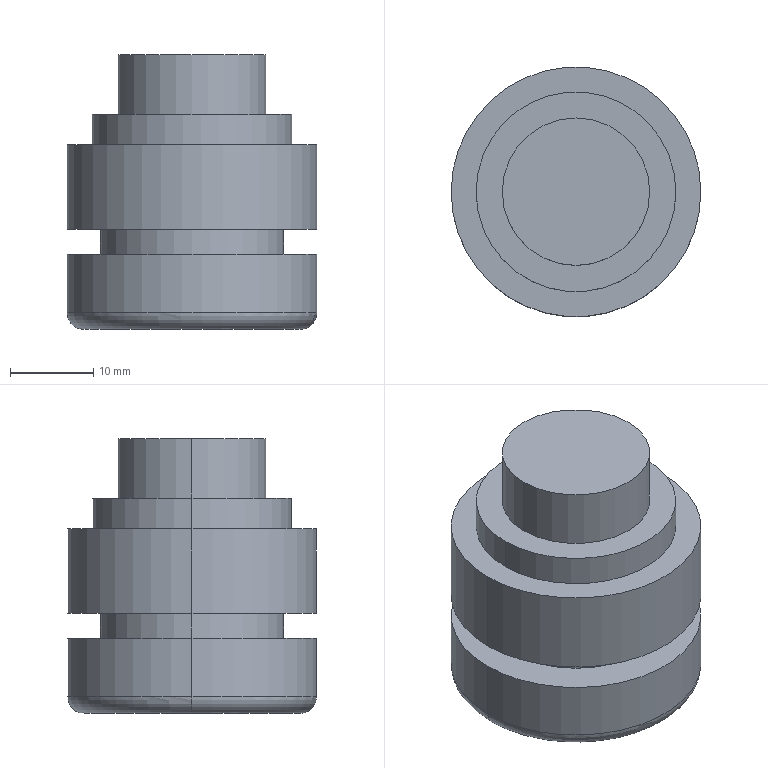Part | STEP file | 1 solid | 18 faces | box 30 x 30 x 33 mm | volume 18043 mm3 | cylinder 10 | plane 6 | torus 2 | commonest cylinder face diameters 30 x4 17.722 x2 22 x2 23.995 x2
STEP:
#1=CARTESIAN_POINT('',(0.,0.,0.));
#2=DIRECTION('',(0.,0.,1.));
#3=DIRECTION('',(1.,0.,0.));
#4=AXIS2_PLACEMENT_3D('',#1,#2,#3);
#5=CARTESIAN_POINT('',(13.,0.,0.));
#6=VERTEX_POINT('',#5);
#7=CARTESIAN_POINT('',(-13.,0.,0.));
#8=VERTEX_POINT('',#7);
#9=CARTESIAN_POINT('',(0.,0.,0.));
#10=DIRECTION('',(0.,0.,1.));
#11=DIRECTION('',(1.,0.,0.));
#12=AXIS2_PLACEMENT_3D('',#9,#10,#11);
#13=CIRCLE('',#12,13.);
#14=CARTESIAN_POINT('',(0.,0.,2.));
#15=DIRECTION('',(0.,0.,1.));
#16=DIRECTION('',(1.,0.,0.));
#17=AXIS2_PLACEMENT_3D('',#14,#15,#16);
#18=TOROIDAL_SURFACE('',#17,13.,2.);
#19=CARTESIAN_POINT('',(0.,4.712));
#20=DIRECTION('',(1.,0.));
#21=VECTOR('',#20,1.);
#22=LINE('',#19,#21);
#23=(GEOMETRIC_REPRESENTATION_CONTEXT(2)PARAMETRIC_REPRESENTATION_CONTEXT()REPRESENTATION_CONTEXT('',''));
#24=DEFINITIONAL_REPRESENTATION('',(#22),#23);
#25=PCURVE('',#18,#24);
#26=CARTESIAN_POINT('',(0.,0.,0.));
#27=DIRECTION('',(0.,0.,-1.));
#28=DIRECTION('',(-1.,0.,0.));
#29=AXIS2_PLACEMENT_3D('',#26,#27,#28);
#30=PLANE('',#29);
#31=CARTESIAN_POINT('',(-13.,0.));
#32=CARTESIAN_POINT('',(-13.,22.517));
#33=CARTESIAN_POINT('',(6.5,11.258));
#34=CARTESIAN_POINT('',(26.,0.));
#35=CARTESIAN_POINT('',(6.5,-11.258));
#36=CARTESIAN_POINT('',(-13.,-22.517));
#37=CARTESIAN_POINT('',(-13.,0.));
#38=(BOUNDED_CURVE()B_SPLINE_CURVE(2,(#31,#32,#33,#34,#35,#36,#37),.UNSPECIFIED.,.T.,.F.)B_SPLINE_CURVE_WITH_KNOTS((1,2,2,2,2,1),(-2.094,0.,2.094,4.189,6.283,8.378),.UNSPECIFIED.)CURVE()GEOMETRIC_REPRESENTATION_ITEM()RATIONAL_B_SPLINE_CURVE((1.,0.5,1.,0.5,1.,0.5,1.))REPRESENTATION_ITEM(''));
#39=(GEOMETRIC_REPRESENTATION_CONTEXT(2)PARAMETRIC_REPRESENTATION_CONTEXT()REPRESENTATION_CONTEXT('',''));
#40=DEFINITIONAL_REPRESENTATION('',(#38),#39);
#41=PCURVE('',#30,#40);
#42=SURFACE_CURVE('',#13,(#25,#41),.PCURVE_S1.);
#43=EDGE_CURVE('',#6,#8,#42,.T.);
#44=ORIENTED_EDGE('',*,*,#43,.T.);
#45=CARTESIAN_POINT('',(-15.,0.,2.));
#46=VERTEX_POINT('',#45);
#47=CARTESIAN_POINT('',(-13.,0.,2.));
#48=DIRECTION('',(0.,1.,0.));
#49=DIRECTION('',(-1.,0.,0.));
#50=AXIS2_PLACEMENT_3D('',#47,#48,#49);
#51=CIRCLE('',#50,2.);
#52=CARTESIAN_POINT('',(3.142,0.));
#53=DIRECTION('',(0.,1.));
#54=VECTOR('',#53,1.);
#55=LINE('',#52,#54);
#56=(GEOMETRIC_REPRESENTATION_CONTEXT(2)PARAMETRIC_REPRESENTATION_CONTEXT()REPRESENTATION_CONTEXT('',''));
#57=DEFINITIONAL_REPRESENTATION('',(#55),#56);
#58=PCURVE('',#18,#57);
#59=CARTESIAN_POINT('',(0.,0.,2.));
#60=DIRECTION('',(0.,0.,1.));
#61=DIRECTION('',(1.,0.,0.));
#62=AXIS2_PLACEMENT_3D('',#59,#60,#61);
#63=TOROIDAL_SURFACE('',#62,13.,2.);
#64=CARTESIAN_POINT('',(3.142,0.));
#65=DIRECTION('',(0.,1.));
#66=VECTOR('',#65,1.);
#67=LINE('',#64,#66);
#68=(GEOMETRIC_REPRESENTATION_CONTEXT(2)PARAMETRIC_REPRESENTATION_CONTEXT()REPRESENTATION_CONTEXT('',''));
#69=DEFINITIONAL_REPRESENTATION('',(#67),#68);
#70=PCURVE('',#63,#69);
#71=SURFACE_CURVE('',#51,(#58,#70),.PCURVE_S1.);
#72=EDGE_CURVE('',#8,#46,#71,.T.);
#73=ORIENTED_EDGE('',*,*,#72,.T.);
#74=CARTESIAN_POINT('',(15.,0.,2.));
#75=VERTEX_POINT('',#74);
#76=CARTESIAN_POINT('',(0.,0.,2.));
#77=DIRECTION('',(0.,0.,1.));
#78=DIRECTION('',(1.,0.,0.));
#79=AXIS2_PLACEMENT_3D('',#76,#77,#78);
#80=CIRCLE('',#79,15.);
#81=CARTESIAN_POINT('',(0.,6.283));
#82=DIRECTION('',(1.,0.));
#83=VECTOR('',#82,1.);
#84=LINE('',#81,#83);
#85=(GEOMETRIC_REPRESENTATION_CONTEXT(2)PARAMETRIC_REPRESENTATION_CONTEXT()REPRESENTATION_CONTEXT('',''));
#86=DEFINITIONAL_REPRESENTATION('',(#84),#85);
#87=PCURVE('',#18,#86);
#88=CARTESIAN_POINT('',(0.,0.,33.));
#89=DIRECTION('',(0.,0.,1.));
#90=DIRECTION('',(1.,0.,0.));
#91=AXIS2_PLACEMENT_3D('',#88,#89,#90);
#92=CYLINDRICAL_SURFACE('',#91,15.);
#93=CARTESIAN_POINT('',(0.,-31.));
#94=DIRECTION('',(1.,0.));
#95=VECTOR('',#94,1.);
#96=LINE('',#93,#95);
#97=(GEOMETRIC_REPRESENTATION_CONTEXT(2)PARAMETRIC_REPRESENTATION_CONTEXT()REPRESENTATION_CONTEXT('',''));
#98=DEFINITIONAL_REPRESENTATION('',(#96),#97);
#99=PCURVE('',#92,#98);
#100=SURFACE_CURVE('',#80,(#87,#99),.PCURVE_S1.);
#101=EDGE_CURVE('',#75,#46,#100,.T.);
#102=ORIENTED_EDGE('',*,*,#101,.F.);
#103=CARTESIAN_POINT('',(13.,0.,2.));
#104=DIRECTION('',(0.,-1.,0.));
#105=DIRECTION('',(0.,0.,-1.));
#106=AXIS2_PLACEMENT_3D('',#103,#104,#105);
#107=CIRCLE('',#106,2.);
#108=CARTESIAN_POINT('',(0.,4.712));
#109=DIRECTION('',(0.,1.));
#110=VECTOR('',#109,1.);
#111=LINE('',#108,#110);
#112=(GEOMETRIC_REPRESENTATION_CONTEXT(2)PARAMETRIC_REPRESENTATION_CONTEXT()REPRESENTATION_CONTEXT('',''));
#113=DEFINITIONAL_REPRESENTATION('',(#111),#112);
#114=PCURVE('',#18,#113);
#115=CARTESIAN_POINT('',(6.283,4.712));
#116=DIRECTION('',(0.,1.));
#117=VECTOR('',#116,1.);
#118=LINE('',#115,#117);
#119=(GEOMETRIC_REPRESENTATION_CONTEXT(2)PARAMETRIC_REPRESENTATION_CONTEXT()REPRESENTATION_CONTEXT('',''));
#120=DEFINITIONAL_REPRESENTATION('',(#118),#119);
#121=PCURVE('',#63,#120);
#122=SURFACE_CURVE('',#107,(#114,#121),.PCURVE_S1.);
#123=EDGE_CURVE('',#6,#75,#122,.T.);
#124=ORIENTED_EDGE('',*,*,#123,.F.);
#125=EDGE_LOOP('',(#44,#73,#102,#124));
#126=FACE_BOUND('',#125,.T.);
#127=ADVANCED_FACE('',(#126),#18,.T.);
#128=ORIENTED_EDGE('',*,*,#101,.T.);
#129=CARTESIAN_POINT('',(-15.,0.,9.));
#130=VERTEX_POINT('',#129);
#131=CARTESIAN_POINT('',(-15.,0.,33.));
#132=DIRECTION('',(0.,0.,1.));
#133=VECTOR('',#132,1.);
#134=LINE('',#131,#133);
#135=CARTESIAN_POINT('',(3.142,0.));
#136=DIRECTION('',(0.,1.));
#137=VECTOR('',#136,1.);
#138=LINE('',#135,#137);
#139=(GEOMETRIC_REPRESENTATION_CONTEXT(2)PARAMETRIC_REPRESENTATION_CONTEXT()REPRESENTATION_CONTEXT('',''));
#140=DEFINITIONAL_REPRESENTATION('',(#138),#139);
#141=PCURVE('',#92,#140);
#142=CARTESIAN_POINT('',(0.,0.,33.));
#143=DIRECTION('',(0.,0.,1.));
#144=DIRECTION('',(1.,0.,0.));
#145=AXIS2_PLACEMENT_3D('',#142,#143,#144);
#146=CYLINDRICAL_SURFACE('',#145,15.);
#147=CARTESIAN_POINT('',(3.142,0.));
#148=DIRECTION('',(0.,1.));
#149=VECTOR('',#148,1.);
#150=LINE('',#147,#149);
#151=(GEOMETRIC_REPRESENTATION_CONTEXT(2)PARAMETRIC_REPRESENTATION_CONTEXT()REPRESENTATION_CONTEXT('',''));
#152=DEFINITIONAL_REPRESENTATION('',(#150),#151);
#153=PCURVE('',#146,#152);
#154=SURFACE_CURVE('',#134,(#141,#153),.PCURVE_S1.);
#155=EDGE_CURVE('',#46,#130,#154,.T.);
#156=ORIENTED_EDGE('',*,*,#155,.T.);
#157=CARTESIAN_POINT('',(15.,0.,9.));
#158=VERTEX_POINT('',#157);
#159=CARTESIAN_POINT('',(0.,0.,9.));
#160=DIRECTION('',(0.,0.,1.));
#161=DIRECTION('',(1.,0.,0.));
#162=AXIS2_PLACEMENT_3D('',#159,#160,#161);
#163=CIRCLE('',#162,15.);
#164=CARTESIAN_POINT('',(0.,-24.));
#165=DIRECTION('',(1.,0.));
#166=VECTOR('',#165,1.);
#167=LINE('',#164,#166);
#168=(GEOMETRIC_REPRESENTATION_CONTEXT(2)PARAMETRIC_REPRESENTATION_CONTEXT()REPRESENTATION_CONTEXT('',''));
#169=DEFINITIONAL_REPRESENTATION('',(#167),#168);
#170=PCURVE('',#92,#169);
#171=CARTESIAN_POINT('',(15.,0.,9.));
#172=DIRECTION('',(0.,0.,1.));
#173=DIRECTION('',(1.,0.,0.));
#174=AXIS2_PLACEMENT_3D('',#171,#172,#173);
#175=PLANE('',#174);
#176=CARTESIAN_POINT('',(-15.,0.));
#177=DIRECTION('',(1.,0.));
#178=AXIS2_PLACEMENT_2D('',#176,#177);
#179=CIRCLE('',#178,15.);
#180=(GEOMETRIC_REPRESENTATION_CONTEXT(2)PARAMETRIC_REPRESENTATION_CONTEXT()REPRESENTATION_CONTEXT('',''));
#181=DEFINITIONAL_REPRESENTATION('',(#179),#180);
#182=PCURVE('',#175,#181);
#183=SURFACE_CURVE('',#163,(#170,#182),.PCURVE_S1.);
#184=EDGE_CURVE('',#158,#130,#183,.T.);
#185=ORIENTED_EDGE('',*,*,#184,.F.);
#186=CARTESIAN_POINT('',(15.,0.,33.));
#187=DIRECTION('',(0.,0.,1.));
#188=VECTOR('',#187,1.);
#189=LINE('',#186,#188);
#190=CARTESIAN_POINT('',(0.,0.));
#191=DIRECTION('',(0.,1.));
#192=VECTOR('',#191,1.);
#193=LINE('',#190,#192);
#194=(GEOMETRIC_REPRESENTATION_CONTEXT(2)PARAMETRIC_REPRESENTATION_CONTEXT()REPRESENTATION_CONTEXT('',''));
#195=DEFINITIONAL_REPRESENTATION('',(#193),#194);
#196=PCURVE('',#92,#195);
#197=CARTESIAN_POINT('',(6.283,0.));
#198=DIRECTION('',(0.,1.));
#199=VECTOR('',#198,1.);
#200=LINE('',#197,#199);
#201=(GEOMETRIC_REPRESENTATION_CONTEXT(2)PARAMETRIC_REPRESENTATION_CONTEXT()REPRESENTATION_CONTEXT('',''));
#202=DEFINITIONAL_REPRESENTATION('',(#200),#201);
#203=PCURVE('',#146,#202);
#204=SURFACE_CURVE('',#189,(#196,#203),.PCURVE_S1.);
#205=EDGE_CURVE('',#75,#158,#204,.T.);
#206=ORIENTED_EDGE('',*,*,#205,.F.);
#207=EDGE_LOOP('',(#128,#156,#185,#206));
#208=FACE_BOUND('',#207,.T.);
#209=ADVANCED_FACE('',(#208),#92,.T.);
#210=CARTESIAN_POINT('',(11.,0.,9.));
#211=VERTEX_POINT('',#210);
#212=CARTESIAN_POINT('',(-11.,0.,9.));
#213=VERTEX_POINT('',#212);
#214=CARTESIAN_POINT('',(0.,0.,9.));
#215=DIRECTION('',(0.,0.,1.));
#216=DIRECTION('',(1.,0.,0.));
#217=AXIS2_PLACEMENT_3D('',#214,#215,#216);
#218=CIRCLE('',#217,11.);
#219=CARTESIAN_POINT('',(0.,0.,33.));
#220=DIRECTION('',(0.,0.,1.));
#221=DIRECTION('',(1.,0.,0.));
#222=AXIS2_PLACEMENT_3D('',#219,#220,#221);
#223=CYLINDRICAL_SURFACE('',#222,11.);
#224=CARTESIAN_POINT('',(0.,-24.));
#225=DIRECTION('',(1.,0.));
#226=VECTOR('',#225,1.);
#227=LINE('',#224,#226);
#228=(GEOMETRIC_REPRESENTATION_CONTEXT(2)PARAMETRIC_REPRESENTATION_CONTEXT()REPRESENTATION_CONTEXT('',''));
#229=DEFINITIONAL_REPRESENTATION('',(#227),#228);
#230=PCURVE('',#223,#229);
#231=CARTESIAN_POINT('',(-15.,0.));
#232=DIRECTION('',(1.,0.));
#233=AXIS2_PLACEMENT_2D('',#231,#232);
#234=CIRCLE('',#233,11.);
#235=(GEOMETRIC_REPRESENTATION_CONTEXT(2)PARAMETRIC_REPRESENTATION_CONTEXT()REPRESENTATION_CONTEXT('',''));
#236=DEFINITIONAL_REPRESENTATION('',(#234),#235);
#237=PCURVE('',#175,#236);
#238=SURFACE_CURVE('',#218,(#230,#237),.PCURVE_S1.);
#239=EDGE_CURVE('',#211,#213,#238,.T.);
#240=ORIENTED_EDGE('',*,*,#239,.T.);
#241=CARTESIAN_POINT('',(-11.,0.,12.));
#242=VERTEX_POINT('',#241);
#243=CARTESIAN_POINT('',(-11.,0.,33.));
#244=DIRECTION('',(0.,0.,1.));
#245=VECTOR('',#244,1.);
#246=LINE('',#243,#245);
#247=CARTESIAN_POINT('',(3.142,0.));
#248=DIRECTION('',(0.,1.));
#249=VECTOR('',#248,1.);
#250=LINE('',#247,#249);
#251=(GEOMETRIC_REPRESENTATION_CONTEXT(2)PARAMETRIC_REPRESENTATION_CONTEXT()REPRESENTATION_CONTEXT('',''));
#252=DEFINITIONAL_REPRESENTATION('',(#250),#251);
#253=PCURVE('',#223,#252);
#254=CARTESIAN_POINT('',(0.,0.,33.));
#255=DIRECTION('',(0.,0.,1.));
#256=DIRECTION('',(1.,0.,0.));
#257=AXIS2_PLACEMENT_3D('',#254,#255,#256);
#258=CYLINDRICAL_SURFACE('',#257,11.);
#259=CARTESIAN_POINT('',(3.142,0.));
#260=DIRECTION('',(0.,1.));
#261=VECTOR('',#260,1.);
#262=LINE('',#259,#261);
#263=(GEOMETRIC_REPRESENTATION_CONTEXT(2)PARAMETRIC_REPRESENTATION_CONTEXT()REPRESENTATION_CONTEXT('',''));
#264=DEFINITIONAL_REPRESENTATION('',(#262),#263);
#265=PCURVE('',#258,#264);
#266=SURFACE_CURVE('',#246,(#253,#265),.PCURVE_S1.);
#267=EDGE_CURVE('',#213,#242,#266,.T.);
#268=ORIENTED_EDGE('',*,*,#267,.T.);
#269=CARTESIAN_POINT('',(11.,0.,12.));
#270=VERTEX_POINT('',#269);
#271=CARTESIAN_POINT('',(0.,0.,12.));
#272=DIRECTION('',(0.,0.,1.));
#273=DIRECTION('',(1.,0.,0.));
#274=AXIS2_PLACEMENT_3D('',#271,#272,#273);
#275=CIRCLE('',#274,11.);
#276=CARTESIAN_POINT('',(0.,-21.));
#277=DIRECTION('',(1.,0.));
#278=VECTOR('',#277,1.);
#279=LINE('',#276,#278);
#280=(GEOMETRIC_REPRESENTATION_CONTEXT(2)PARAMETRIC_REPRESENTATION_CONTEXT()REPRESENTATION_CONTEXT('',''));
#281=DEFINITIONAL_REPRESENTATION('',(#279),#280);
#282=PCURVE('',#223,#281);
#283=CARTESIAN_POINT('',(11.,0.,12.));
#284=DIRECTION('',(0.,0.,-1.));
#285=DIRECTION('',(-1.,0.,0.));
#286=AXIS2_PLACEMENT_3D('',#283,#284,#285);
#287=PLANE('',#286);
#288=CARTESIAN_POINT('',(0.,0.));
#289=CARTESIAN_POINT('',(0.,19.053));
#290=CARTESIAN_POINT('',(16.5,9.526));
#291=CARTESIAN_POINT('',(33.,0.));
#292=CARTESIAN_POINT('',(16.5,-9.526));
#293=CARTESIAN_POINT('',(0.,-19.053));
#294=CARTESIAN_POINT('',(0.,0.));
#295=(BOUNDED_CURVE()B_SPLINE_CURVE(2,(#288,#289,#290,#291,#292,#293,#294),.UNSPECIFIED.,.T.,.F.)B_SPLINE_CURVE_WITH_KNOTS((1,2,2,2,2,1),(-2.094,0.,2.094,4.189,6.283,8.378),.UNSPECIFIED.)CURVE()GEOMETRIC_REPRESENTATION_ITEM()RATIONAL_B_SPLINE_CURVE((1.,0.5,1.,0.5,1.,0.5,1.))REPRESENTATION_ITEM(''));
#296=(GEOMETRIC_REPRESENTATION_CONTEXT(2)PARAMETRIC_REPRESENTATION_CONTEXT()REPRESENTATION_CONTEXT('',''));
#297=DEFINITIONAL_REPRESENTATION('',(#295),#296);
#298=PCURVE('',#287,#297);
#299=SURFACE_CURVE('',#275,(#282,#298),.PCURVE_S1.);
#300=EDGE_CURVE('',#270,#242,#299,.T.);
#301=ORIENTED_EDGE('',*,*,#300,.F.);
#302=CARTESIAN_POINT('',(11.,0.,33.));
#303=DIRECTION('',(0.,0.,1.));
#304=VECTOR('',#303,1.);
#305=LINE('',#302,#304);
#306=CARTESIAN_POINT('',(0.,0.));
#307=DIRECTION('',(0.,1.));
#308=VECTOR('',#307,1.);
#309=LINE('',#306,#308);
#310=(GEOMETRIC_REPRESENTATION_CONTEXT(2)PARAMETRIC_REPRESENTATION_CONTEXT()REPRESENTATION_CONTEXT('',''));
#311=DEFINITIONAL_REPRESENTATION('',(#309),#310);
#312=PCURVE('',#223,#311);
#313=CARTESIAN_POINT('',(6.283,0.));
#314=DIRECTION('',(0.,1.));
#315=VECTOR('',#314,1.);
#316=LINE('',#313,#315);
#317=(GEOMETRIC_REPRESENTATION_CONTEXT(2)PARAMETRIC_REPRESENTATION_CONTEXT()REPRESENTATION_CONTEXT('',''));
#318=DEFINITIONAL_REPRESENTATION('',(#316),#317);
#319=PCURVE('',#258,#318);
#320=SURFACE_CURVE('',#305,(#312,#319),.PCURVE_S1.);
#321=EDGE_CURVE('',#211,#270,#320,.T.);
#322=ORIENTED_EDGE('',*,*,#321,.F.);
#323=EDGE_LOOP('',(#240,#268,#301,#322));
#324=FACE_BOUND('',#323,.T.);
#325=ADVANCED_FACE('',(#324),#223,.T.);
#326=CARTESIAN_POINT('',(15.,0.,12.));
#327=VERTEX_POINT('',#326);
#328=CARTESIAN_POINT('',(-15.,0.,12.));
#329=VERTEX_POINT('',#328);
#330=CARTESIAN_POINT('',(0.,0.,12.));
#331=DIRECTION('',(0.,0.,1.));
#332=DIRECTION('',(1.,0.,0.));
#333=AXIS2_PLACEMENT_3D('',#330,#331,#332);
#334=CIRCLE('',#333,15.);
#335=CARTESIAN_POINT('',(0.,0.,33.));
#336=DIRECTION('',(0.,0.,1.));
#337=DIRECTION('',(1.,0.,0.));
#338=AXIS2_PLACEMENT_3D('',#335,#336,#337);
#339=CYLINDRICAL_SURFACE('',#338,15.);
#340=CARTESIAN_POINT('',(0.,-21.));
#341=DIRECTION('',(1.,0.));
#342=VECTOR('',#341,1.);
#343=LINE('',#340,#342);
#344=(GEOMETRIC_REPRESENTATION_CONTEXT(2)PARAMETRIC_REPRESENTATION_CONTEXT()REPRESENTATION_CONTEXT('',''));
#345=DEFINITIONAL_REPRESENTATION('',(#343),#344);
#346=PCURVE('',#339,#345);
#347=CARTESIAN_POINT('',(-4.,0.));
#348=CARTESIAN_POINT('',(-4.,25.981));
#349=CARTESIAN_POINT('',(18.5,12.99));
#350=CARTESIAN_POINT('',(41.,0.));
#351=CARTESIAN_POINT('',(18.5,-12.99));
#352=CARTESIAN_POINT('',(-4.,-25.981));
#353=CARTESIAN_POINT('',(-4.,0.));
#354=(BOUNDED_CURVE()B_SPLINE_CURVE(2,(#347,#348,#349,#350,#351,#352,#353),.UNSPECIFIED.,.T.,.F.)B_SPLINE_CURVE_WITH_KNOTS((1,2,2,2,2,1),(-2.094,0.,2.094,4.189,6.283,8.378),.UNSPECIFIED.)CURVE()GEOMETRIC_REPRESENTATION_ITEM()RATIONAL_B_SPLINE_CURVE((1.,0.5,1.,0.5,1.,0.5,1.))REPRESENTATION_ITEM(''));
#355=(GEOMETRIC_REPRESENTATION_CONTEXT(2)PARAMETRIC_REPRESENTATION_CONTEXT()REPRESENTATION_CONTEXT('',''));
#356=DEFINITIONAL_REPRESENTATION('',(#354),#355);
#357=PCURVE('',#287,#356);
#358=SURFACE_CURVE('',#334,(#346,#357),.PCURVE_S1.);
#359=EDGE_CURVE('',#327,#329,#358,.T.);
#360=ORIENTED_EDGE('',*,*,#359,.T.);
#361=CARTESIAN_POINT('',(-15.,0.,22.166));
#362=VERTEX_POINT('',#361);
#363=CARTESIAN_POINT('',(-15.,0.,33.));
#364=DIRECTION('',(0.,0.,1.));
#365=VECTOR('',#364,1.);
#366=LINE('',#363,#365);
#367=CARTESIAN_POINT('',(3.142,0.));
#368=DIRECTION('',(0.,1.));
#369=VECTOR('',#368,1.);
#370=LINE('',#367,#369);
#371=(GEOMETRIC_REPRESENTATION_CONTEXT(2)PARAMETRIC_REPRESENTATION_CONTEXT()REPRESENTATION_CONTEXT('',''));
#372=DEFINITIONAL_REPRESENTATION('',(#370),#371);
#373=PCURVE('',#339,#372);
#374=CARTESIAN_POINT('',(0.,0.,33.));
#375=DIRECTION('',(0.,0.,1.));
#376=DIRECTION('',(1.,0.,0.));
#377=AXIS2_PLACEMENT_3D('',#374,#375,#376);
#378=CYLINDRICAL_SURFACE('',#377,15.);
#379=CARTESIAN_POINT('',(3.142,0.));
#380=DIRECTION('',(0.,1.));
#381=VECTOR('',#380,1.);
#382=LINE('',#379,#381);
#383=(GEOMETRIC_REPRESENTATION_CONTEXT(2)PARAMETRIC_REPRESENTATION_CONTEXT()REPRESENTATION_CONTEXT('',''));
#384=DEFINITIONAL_REPRESENTATION('',(#382),#383);
#385=PCURVE('',#378,#384);
#386=SURFACE_CURVE('',#366,(#373,#385),.PCURVE_S1.);
#387=EDGE_CURVE('',#329,#362,#386,.T.);
#388=ORIENTED_EDGE('',*,*,#387,.T.);
#389=CARTESIAN_POINT('',(15.,0.,22.166));
#390=VERTEX_POINT('',#389);
#391=CARTESIAN_POINT('',(0.,0.,22.166));
#392=DIRECTION('',(0.,0.,1.));
#393=DIRECTION('',(1.,0.,0.));
#394=AXIS2_PLACEMENT_3D('',#391,#392,#393);
#395=CIRCLE('',#394,15.);
#396=CARTESIAN_POINT('',(0.,-10.834));
#397=DIRECTION('',(1.,0.));
#398=VECTOR('',#397,1.);
#399=LINE('',#396,#398);
#400=(GEOMETRIC_REPRESENTATION_CONTEXT(2)PARAMETRIC_REPRESENTATION_CONTEXT()REPRESENTATION_CONTEXT('',''));
#401=DEFINITIONAL_REPRESENTATION('',(#399),#400);
#402=PCURVE('',#339,#401);
#403=CARTESIAN_POINT('',(15.,0.,22.166));
#404=DIRECTION('',(0.,0.,1.));
#405=DIRECTION('',(1.,0.,0.));
#406=AXIS2_PLACEMENT_3D('',#403,#404,#405);
#407=PLANE('',#406);
#408=CARTESIAN_POINT('',(-15.,0.));
#409=DIRECTION('',(1.,0.));
#410=AXIS2_PLACEMENT_2D('',#408,#409);
#411=CIRCLE('',#410,15.);
#412=(GEOMETRIC_REPRESENTATION_CONTEXT(2)PARAMETRIC_REPRESENTATION_CONTEXT()REPRESENTATION_CONTEXT('',''));
#413=DEFINITIONAL_REPRESENTATION('',(#411),#412);
#414=PCURVE('',#407,#413);
#415=SURFACE_CURVE('',#395,(#402,#414),.PCURVE_S1.);
#416=EDGE_CURVE('',#390,#362,#415,.T.);
#417=ORIENTED_EDGE('',*,*,#416,.F.);
#418=CARTESIAN_POINT('',(15.,0.,33.));
#419=DIRECTION('',(0.,0.,1.));
#420=VECTOR('',#419,1.);
#421=LINE('',#418,#420);
#422=CARTESIAN_POINT('',(0.,0.));
#423=DIRECTION('',(0.,1.));
#424=VECTOR('',#423,1.);
#425=LINE('',#422,#424);
#426=(GEOMETRIC_REPRESENTATION_CONTEXT(2)PARAMETRIC_REPRESENTATION_CONTEXT()REPRESENTATION_CONTEXT('',''));
#427=DEFINITIONAL_REPRESENTATION('',(#425),#426);
#428=PCURVE('',#339,#427);
#429=CARTESIAN_POINT('',(6.283,0.));
#430=DIRECTION('',(0.,1.));
#431=VECTOR('',#430,1.);
#432=LINE('',#429,#431);
#433=(GEOMETRIC_REPRESENTATION_CONTEXT(2)PARAMETRIC_REPRESENTATION_CONTEXT()REPRESENTATION_CONTEXT('',''));
#434=DEFINITIONAL_REPRESENTATION('',(#432),#433);
#435=PCURVE('',#378,#434);
#436=SURFACE_CURVE('',#421,(#428,#435),.PCURVE_S1.);
#437=EDGE_CURVE('',#327,#390,#436,.T.);
#438=ORIENTED_EDGE('',*,*,#437,.F.);
#439=EDGE_LOOP('',(#360,#388,#417,#438));
#440=FACE_BOUND('',#439,.T.);
#441=ADVANCED_FACE('',(#440),#339,.T.);
#442=CARTESIAN_POINT('',(11.997,0.,22.166));
#443=VERTEX_POINT('',#442);
#444=CARTESIAN_POINT('',(-11.997,0.,22.166));
#445=VERTEX_POINT('',#444);
#446=CARTESIAN_POINT('',(0.,0.,22.166));
#447=DIRECTION('',(0.,0.,1.));
#448=DIRECTION('',(1.,0.,0.));
#449=AXIS2_PLACEMENT_3D('',#446,#447,#448);
#450=CIRCLE('',#449,11.997);
#451=CARTESIAN_POINT('',(0.,0.,33.));
#452=DIRECTION('',(0.,0.,1.));
#453=DIRECTION('',(1.,0.,0.));
#454=AXIS2_PLACEMENT_3D('',#451,#452,#453);
#455=CYLINDRICAL_SURFACE('',#454,11.997);
#456=CARTESIAN_POINT('',(0.,-10.834));
#457=DIRECTION('',(1.,0.));
#458=VECTOR('',#457,1.);
#459=LINE('',#456,#458);
#460=(GEOMETRIC_REPRESENTATION_CONTEXT(2)PARAMETRIC_REPRESENTATION_CONTEXT()REPRESENTATION_CONTEXT('',''));
#461=DEFINITIONAL_REPRESENTATION('',(#459),#460);
#462=PCURVE('',#455,#461);
#463=CARTESIAN_POINT('',(-15.,0.));
#464=DIRECTION('',(1.,0.));
#465=AXIS2_PLACEMENT_2D('',#463,#464);
#466=CIRCLE('',#465,11.997);
#467=(GEOMETRIC_REPRESENTATION_CONTEXT(2)PARAMETRIC_REPRESENTATION_CONTEXT()REPRESENTATION_CONTEXT('',''));
#468=DEFINITIONAL_REPRESENTATION('',(#466),#467);
#469=PCURVE('',#407,#468);
#470=SURFACE_CURVE('',#450,(#462,#469),.PCURVE_S1.);
#471=EDGE_CURVE('',#443,#445,#470,.T.);
#472=ORIENTED_EDGE('',*,*,#471,.T.);
#473=CARTESIAN_POINT('',(-11.997,0.,25.869));
#474=VERTEX_POINT('',#473);
#475=CARTESIAN_POINT('',(-11.997,0.,33.));
#476=DIRECTION('',(0.,0.,1.));
#477=VECTOR('',#476,1.);
#478=LINE('',#475,#477);
#479=CARTESIAN_POINT('',(3.142,0.));
#480=DIRECTION('',(0.,1.));
#481=VECTOR('',#480,1.);
#482=LINE('',#479,#481);
#483=(GEOMETRIC_REPRESENTATION_CONTEXT(2)PARAMETRIC_REPRESENTATION_CONTEXT()REPRESENTATION_CONTEXT('',''));
#484=DEFINITIONAL_REPRESENTATION('',(#482),#483);
#485=PCURVE('',#455,#484);
#486=CARTESIAN_POINT('',(0.,0.,33.));
#487=DIRECTION('',(0.,0.,1.));
#488=DIRECTION('',(1.,0.,0.));
#489=AXIS2_PLACEMENT_3D('',#486,#487,#488);
#490=CYLINDRICAL_SURFACE('',#489,11.997);
#491=CARTESIAN_POINT('',(3.142,0.));
#492=DIRECTION('',(0.,1.));
#493=VECTOR('',#492,1.);
#494=LINE('',#491,#493);
#495=(GEOMETRIC_REPRESENTATION_CONTEXT(2)PARAMETRIC_REPRESENTATION_CONTEXT()REPRESENTATION_CONTEXT('',''));
#496=DEFINITIONAL_REPRESENTATION('',(#494),#495);
#497=PCURVE('',#490,#496);
#498=SURFACE_CURVE('',#478,(#485,#497),.PCURVE_S1.);
#499=EDGE_CURVE('',#445,#474,#498,.T.);
#500=ORIENTED_EDGE('',*,*,#499,.T.);
#501=CARTESIAN_POINT('',(11.997,0.,25.869));
#502=VERTEX_POINT('',#501);
#503=CARTESIAN_POINT('',(0.,0.,25.869));
#504=DIRECTION('',(0.,0.,1.));
#505=DIRECTION('',(1.,0.,0.));
#506=AXIS2_PLACEMENT_3D('',#503,#504,#505);
#507=CIRCLE('',#506,11.997);
#508=CARTESIAN_POINT('',(0.,-7.131));
#509=DIRECTION('',(1.,0.));
#510=VECTOR('',#509,1.);
#511=LINE('',#508,#510);
#512=(GEOMETRIC_REPRESENTATION_CONTEXT(2)PARAMETRIC_REPRESENTATION_CONTEXT()REPRESENTATION_CONTEXT('',''));
#513=DEFINITIONAL_REPRESENTATION('',(#511),#512);
#514=PCURVE('',#455,#513);
#515=CARTESIAN_POINT('',(11.997,0.,25.869));
#516=DIRECTION('',(0.,0.,1.));
#517=DIRECTION('',(1.,0.,0.));
#518=AXIS2_PLACEMENT_3D('',#515,#516,#517);
#519=PLANE('',#518);
#520=CARTESIAN_POINT('',(-11.997,0.));
#521=DIRECTION('',(1.,0.));
#522=AXIS2_PLACEMENT_2D('',#520,#521);
#523=CIRCLE('',#522,11.997);
#524=(GEOMETRIC_REPRESENTATION_CONTEXT(2)PARAMETRIC_REPRESENTATION_CONTEXT()REPRESENTATION_CONTEXT('',''));
#525=DEFINITIONAL_REPRESENTATION('',(#523),#524);
#526=PCURVE('',#519,#525);
#527=SURFACE_CURVE('',#507,(#514,#526),.PCURVE_S1.);
#528=EDGE_CURVE('',#502,#474,#527,.T.);
#529=ORIENTED_EDGE('',*,*,#528,.F.);
#530=CARTESIAN_POINT('',(11.997,0.,33.));
#531=DIRECTION('',(0.,0.,1.));
#532=VECTOR('',#531,1.);
#533=LINE('',#530,#532);
#534=CARTESIAN_POINT('',(0.,0.));
#535=DIRECTION('',(0.,1.));
#536=VECTOR('',#535,1.);
#537=LINE('',#534,#536);
#538=(GEOMETRIC_REPRESENTATION_CONTEXT(2)PARAMETRIC_REPRESENTATION_CONTEXT()REPRESENTATION_CONTEXT('',''));
#539=DEFINITIONAL_REPRESENTATION('',(#537),#538);
#540=PCURVE('',#455,#539);
#541=CARTESIAN_POINT('',(6.283,0.));
#542=DIRECTION('',(0.,1.));
#543=VECTOR('',#542,1.);
#544=LINE('',#541,#543);
#545=(GEOMETRIC_REPRESENTATION_CONTEXT(2)PARAMETRIC_REPRESENTATION_CONTEXT()REPRESENTATION_CONTEXT('',''));
#546=DEFINITIONAL_REPRESENTATION('',(#544),#545);
#547=PCURVE('',#490,#546);
#548=SURFACE_CURVE('',#533,(#540,#547),.PCURVE_S1.);
#549=EDGE_CURVE('',#443,#502,#548,.T.);
#550=ORIENTED_EDGE('',*,*,#549,.F.);
#551=EDGE_LOOP('',(#472,#500,#529,#550));
#552=FACE_BOUND('',#551,.T.);
#553=ADVANCED_FACE('',(#552),#455,.T.);
#554=CARTESIAN_POINT('',(8.861,0.,25.869));
#555=VERTEX_POINT('',#554);
#556=CARTESIAN_POINT('',(-8.861,0.,25.869));
#557=VERTEX_POINT('',#556);
#558=CARTESIAN_POINT('',(0.,0.,25.869));
#559=DIRECTION('',(0.,0.,1.));
#560=DIRECTION('',(1.,0.,0.));
#561=AXIS2_PLACEMENT_3D('',#558,#559,#560);
#562=CIRCLE('',#561,8.861);
#563=CARTESIAN_POINT('',(0.,0.,33.));
#564=DIRECTION('',(0.,0.,1.));
#565=DIRECTION('',(1.,0.,0.));
#566=AXIS2_PLACEMENT_3D('',#563,#564,#565);
#567=CYLINDRICAL_SURFACE('',#566,8.861);
#568=CARTESIAN_POINT('',(0.,-7.131));
#569=DIRECTION('',(1.,0.));
#570=VECTOR('',#569,1.);
#571=LINE('',#568,#570);
#572=(GEOMETRIC_REPRESENTATION_CONTEXT(2)PARAMETRIC_REPRESENTATION_CONTEXT()REPRESENTATION_CONTEXT('',''));
#573=DEFINITIONAL_REPRESENTATION('',(#571),#572);
#574=PCURVE('',#567,#573);
#575=CARTESIAN_POINT('',(-11.997,0.));
#576=DIRECTION('',(1.,0.));
#577=AXIS2_PLACEMENT_2D('',#575,#576);
#578=CIRCLE('',#577,8.861);
#579=(GEOMETRIC_REPRESENTATION_CONTEXT(2)PARAMETRIC_REPRESENTATION_CONTEXT()REPRESENTATION_CONTEXT('',''));
#580=DEFINITIONAL_REPRESENTATION('',(#578),#579);
#581=PCURVE('',#519,#580);
#582=SURFACE_CURVE('',#562,(#574,#581),.PCURVE_S1.);
#583=EDGE_CURVE('',#555,#557,#582,.T.);
#584=ORIENTED_EDGE('',*,*,#583,.T.);
#585=CARTESIAN_POINT('',(-8.861,0.,33.));
#586=VERTEX_POINT('',#585);
#587=CARTESIAN_POINT('',(-8.861,0.,33.));
#588=DIRECTION('',(0.,0.,1.));
#589=VECTOR('',#588,1.);
#590=LINE('',#587,#589);
#591=CARTESIAN_POINT('',(3.142,0.));
#592=DIRECTION('',(0.,1.));
#593=VECTOR('',#592,1.);
#594=LINE('',#591,#593);
#595=(GEOMETRIC_REPRESENTATION_CONTEXT(2)PARAMETRIC_REPRESENTATION_CONTEXT()REPRESENTATION_CONTEXT('',''));
#596=DEFINITIONAL_REPRESENTATION('',(#594),#595);
#597=PCURVE('',#567,#596);
#598=CARTESIAN_POINT('',(0.,0.,33.));
#599=DIRECTION('',(0.,0.,1.));
#600=DIRECTION('',(1.,0.,0.));
#601=AXIS2_PLACEMENT_3D('',#598,#599,#600);
#602=CYLINDRICAL_SURFACE('',#601,8.861);
#603=CARTESIAN_POINT('',(3.142,0.));
#604=DIRECTION('',(0.,1.));
#605=VECTOR('',#604,1.);
#606=LINE('',#603,#605);
#607=(GEOMETRIC_REPRESENTATION_CONTEXT(2)PARAMETRIC_REPRESENTATION_CONTEXT()REPRESENTATION_CONTEXT('',''));
#608=DEFINITIONAL_REPRESENTATION('',(#606),#607);
#609=PCURVE('',#602,#608);
#610=SURFACE_CURVE('',#590,(#597,#609),.PCURVE_S1.);
#611=EDGE_CURVE('',#557,#586,#610,.T.);
#612=ORIENTED_EDGE('',*,*,#611,.T.);
#613=CARTESIAN_POINT('',(8.861,0.,33.));
#614=VERTEX_POINT('',#613);
#615=CARTESIAN_POINT('',(0.,0.,33.));
#616=DIRECTION('',(0.,0.,1.));
#617=DIRECTION('',(1.,0.,0.));
#618=AXIS2_PLACEMENT_3D('',#615,#616,#617);
#619=CIRCLE('',#618,8.861);
#620=CARTESIAN_POINT('',(0.,0.));
#621=DIRECTION('',(1.,0.));
#622=VECTOR('',#621,1.);
#623=LINE('',#620,#622);
#624=(GEOMETRIC_REPRESENTATION_CONTEXT(2)PARAMETRIC_REPRESENTATION_CONTEXT()REPRESENTATION_CONTEXT('',''));
#625=DEFINITIONAL_REPRESENTATION('',(#623),#624);
#626=PCURVE('',#567,#625);
#627=CARTESIAN_POINT('',(8.861,0.,33.));
#628=DIRECTION('',(0.,0.,1.));
#629=DIRECTION('',(1.,0.,0.));
#630=AXIS2_PLACEMENT_3D('',#627,#628,#629);
#631=PLANE('',#630);
#632=CARTESIAN_POINT('',(-8.861,0.));
#633=DIRECTION('',(1.,0.));
#634=AXIS2_PLACEMENT_2D('',#632,#633);
#635=CIRCLE('',#634,8.861);
#636=(GEOMETRIC_REPRESENTATION_CONTEXT(2)PARAMETRIC_REPRESENTATION_CONTEXT()REPRESENTATION_CONTEXT('',''));
#637=DEFINITIONAL_REPRESENTATION('',(#635),#636);
#638=PCURVE('',#631,#637);
#639=SURFACE_CURVE('',#619,(#626,#638),.PCURVE_S1.);
#640=EDGE_CURVE('',#614,#586,#639,.T.);
#641=ORIENTED_EDGE('',*,*,#640,.F.);
#642=CARTESIAN_POINT('',(8.861,0.,33.));
#643=DIRECTION('',(0.,0.,1.));
#644=VECTOR('',#643,1.);
#645=LINE('',#642,#644);
#646=CARTESIAN_POINT('',(0.,0.));
#647=DIRECTION('',(0.,1.));
#648=VECTOR('',#647,1.);
#649=LINE('',#646,#648);
#650=(GEOMETRIC_REPRESENTATION_CONTEXT(2)PARAMETRIC_REPRESENTATION_CONTEXT()REPRESENTATION_CONTEXT('',''));
#651=DEFINITIONAL_REPRESENTATION('',(#649),#650);
#652=PCURVE('',#567,#651);
#653=CARTESIAN_POINT('',(6.283,0.));
#654=DIRECTION('',(0.,1.));
#655=VECTOR('',#654,1.);
#656=LINE('',#653,#655);
#657=(GEOMETRIC_REPRESENTATION_CONTEXT(2)PARAMETRIC_REPRESENTATION_CONTEXT()REPRESENTATION_CONTEXT('',''));
#658=DEFINITIONAL_REPRESENTATION('',(#656),#657);
#659=PCURVE('',#602,#658);
#660=SURFACE_CURVE('',#645,(#652,#659),.PCURVE_S1.);
#661=EDGE_CURVE('',#555,#614,#660,.T.);
#662=ORIENTED_EDGE('',*,*,#661,.F.);
#663=EDGE_LOOP('',(#584,#612,#641,#662));
#664=FACE_BOUND('',#663,.T.);
#665=ADVANCED_FACE('',(#664),#567,.T.);
#666=ORIENTED_EDGE('',*,*,#640,.T.);
#667=CARTESIAN_POINT('',(0.,0.,33.));
#668=DIRECTION('',(0.,0.,1.));
#669=DIRECTION('',(1.,0.,0.));
#670=AXIS2_PLACEMENT_3D('',#667,#668,#669);
#671=CIRCLE('',#670,8.861);
#672=CARTESIAN_POINT('',(-8.861,0.));
#673=DIRECTION('',(1.,0.));
#674=AXIS2_PLACEMENT_2D('',#672,#673);
#675=CIRCLE('',#674,8.861);
#676=(GEOMETRIC_REPRESENTATION_CONTEXT(2)PARAMETRIC_REPRESENTATION_CONTEXT()REPRESENTATION_CONTEXT('',''));
#677=DEFINITIONAL_REPRESENTATION('',(#675),#676);
#678=PCURVE('',#631,#677);
#679=CARTESIAN_POINT('',(0.,0.));
#680=DIRECTION('',(1.,0.));
#681=VECTOR('',#680,1.);
#682=LINE('',#679,#681);
#683=(GEOMETRIC_REPRESENTATION_CONTEXT(2)PARAMETRIC_REPRESENTATION_CONTEXT()REPRESENTATION_CONTEXT('',''));
#684=DEFINITIONAL_REPRESENTATION('',(#682),#683);
#685=PCURVE('',#602,#684);
#686=SURFACE_CURVE('',#671,(#678,#685),.PCURVE_S1.);
#687=EDGE_CURVE('',#586,#614,#686,.T.);
#688=ORIENTED_EDGE('',*,*,#687,.T.);
#689=EDGE_LOOP('',(#666,#688));
#690=FACE_BOUND('',#689,.T.);
#691=ADVANCED_FACE('',(#690),#631,.T.);
#692=ORIENTED_EDGE('',*,*,#611,.F.);
#693=CARTESIAN_POINT('',(0.,0.,25.869));
#694=DIRECTION('',(0.,0.,1.));
#695=DIRECTION('',(1.,0.,0.));
#696=AXIS2_PLACEMENT_3D('',#693,#694,#695);
#697=CIRCLE('',#696,8.861);
#698=CARTESIAN_POINT('',(0.,-7.131));
#699=DIRECTION('',(1.,0.));
#700=VECTOR('',#699,1.);
#701=LINE('',#698,#700);
#702=(GEOMETRIC_REPRESENTATION_CONTEXT(2)PARAMETRIC_REPRESENTATION_CONTEXT()REPRESENTATION_CONTEXT('',''));
#703=DEFINITIONAL_REPRESENTATION('',(#701),#702);
#704=PCURVE('',#602,#703);
#705=CARTESIAN_POINT('',(-11.997,0.));
#706=DIRECTION('',(1.,0.));
#707=AXIS2_PLACEMENT_2D('',#705,#706);
#708=CIRCLE('',#707,8.861);
#709=(GEOMETRIC_REPRESENTATION_CONTEXT(2)PARAMETRIC_REPRESENTATION_CONTEXT()REPRESENTATION_CONTEXT('',''));
#710=DEFINITIONAL_REPRESENTATION('',(#708),#709);
#711=PCURVE('',#519,#710);
#712=SURFACE_CURVE('',#697,(#704,#711),.PCURVE_S1.);
#713=EDGE_CURVE('',#557,#555,#712,.T.);
#714=ORIENTED_EDGE('',*,*,#713,.T.);
#715=ORIENTED_EDGE('',*,*,#661,.T.);
#716=ORIENTED_EDGE('',*,*,#687,.F.);
#717=EDGE_LOOP('',(#692,#714,#715,#716));
#718=FACE_BOUND('',#717,.T.);
#719=ADVANCED_FACE('',(#718),#602,.T.);
#720=ORIENTED_EDGE('',*,*,#528,.T.);
#721=CARTESIAN_POINT('',(0.,0.,25.869));
#722=DIRECTION('',(0.,0.,1.));
#723=DIRECTION('',(1.,0.,0.));
#724=AXIS2_PLACEMENT_3D('',#721,#722,#723);
#725=CIRCLE('',#724,11.997);
#726=CARTESIAN_POINT('',(-11.997,0.));
#727=DIRECTION('',(1.,0.));
#728=AXIS2_PLACEMENT_2D('',#726,#727);
#729=CIRCLE('',#728,11.997);
#730=(GEOMETRIC_REPRESENTATION_CONTEXT(2)PARAMETRIC_REPRESENTATION_CONTEXT()REPRESENTATION_CONTEXT('',''));
#731=DEFINITIONAL_REPRESENTATION('',(#729),#730);
#732=PCURVE('',#519,#731);
#733=CARTESIAN_POINT('',(0.,-7.131));
#734=DIRECTION('',(1.,0.));
#735=VECTOR('',#734,1.);
#736=LINE('',#733,#735);
#737=(GEOMETRIC_REPRESENTATION_CONTEXT(2)PARAMETRIC_REPRESENTATION_CONTEXT()REPRESENTATION_CONTEXT('',''));
#738=DEFINITIONAL_REPRESENTATION('',(#736),#737);
#739=PCURVE('',#490,#738);
#740=SURFACE_CURVE('',#725,(#732,#739),.PCURVE_S1.);
#741=EDGE_CURVE('',#474,#502,#740,.T.);
#742=ORIENTED_EDGE('',*,*,#741,.T.);
#743=EDGE_LOOP('',(#720,#742));
#744=FACE_BOUND('',#743,.T.);
#745=ORIENTED_EDGE('',*,*,#583,.F.);
#746=ORIENTED_EDGE('',*,*,#713,.F.);
#747=EDGE_LOOP('',(#745,#746));
#748=FACE_BOUND('',#747,.T.);
#749=ADVANCED_FACE('',(#744,#748),#519,.T.);
#750=ORIENTED_EDGE('',*,*,#499,.F.);
#751=CARTESIAN_POINT('',(0.,0.,22.166));
#752=DIRECTION('',(0.,0.,1.));
#753=DIRECTION('',(1.,0.,0.));
#754=AXIS2_PLACEMENT_3D('',#751,#752,#753);
#755=CIRCLE('',#754,11.997);
#756=CARTESIAN_POINT('',(0.,-10.834));
#757=DIRECTION('',(1.,0.));
#758=VECTOR('',#757,1.);
#759=LINE('',#756,#758);
#760=(GEOMETRIC_REPRESENTATION_CONTEXT(2)PARAMETRIC_REPRESENTATION_CONTEXT()REPRESENTATION_CONTEXT('',''));
#761=DEFINITIONAL_REPRESENTATION('',(#759),#760);
#762=PCURVE('',#490,#761);
#763=CARTESIAN_POINT('',(-15.,0.));
#764=DIRECTION('',(1.,0.));
#765=AXIS2_PLACEMENT_2D('',#763,#764);
#766=CIRCLE('',#765,11.997);
#767=(GEOMETRIC_REPRESENTATION_CONTEXT(2)PARAMETRIC_REPRESENTATION_CONTEXT()REPRESENTATION_CONTEXT('',''));
#768=DEFINITIONAL_REPRESENTATION('',(#766),#767);
#769=PCURVE('',#407,#768);
#770=SURFACE_CURVE('',#755,(#762,#769),.PCURVE_S1.);
#771=EDGE_CURVE('',#445,#443,#770,.T.);
#772=ORIENTED_EDGE('',*,*,#771,.T.);
#773=ORIENTED_EDGE('',*,*,#549,.T.);
#774=ORIENTED_EDGE('',*,*,#741,.F.);
#775=EDGE_LOOP('',(#750,#772,#773,#774));
#776=FACE_BOUND('',#775,.T.);
#777=ADVANCED_FACE('',(#776),#490,.T.);
#778=ORIENTED_EDGE('',*,*,#416,.T.);
#779=CARTESIAN_POINT('',(0.,0.,22.166));
#780=DIRECTION('',(0.,0.,1.));
#781=DIRECTION('',(1.,0.,0.));
#782=AXIS2_PLACEMENT_3D('',#779,#780,#781);
#783=CIRCLE('',#782,15.);
#784=CARTESIAN_POINT('',(-15.,0.));
#785=DIRECTION('',(1.,0.));
#786=AXIS2_PLACEMENT_2D('',#784,#785);
#787=CIRCLE('',#786,15.);
#788=(GEOMETRIC_REPRESENTATION_CONTEXT(2)PARAMETRIC_REPRESENTATION_CONTEXT()REPRESENTATION_CONTEXT('',''));
#789=DEFINITIONAL_REPRESENTATION('',(#787),#788);
#790=PCURVE('',#407,#789);
#791=CARTESIAN_POINT('',(0.,-10.834));
#792=DIRECTION('',(1.,0.));
#793=VECTOR('',#792,1.);
#794=LINE('',#791,#793);
#795=(GEOMETRIC_REPRESENTATION_CONTEXT(2)PARAMETRIC_REPRESENTATION_CONTEXT()REPRESENTATION_CONTEXT('',''));
#796=DEFINITIONAL_REPRESENTATION('',(#794),#795);
#797=PCURVE('',#378,#796);
#798=SURFACE_CURVE('',#783,(#790,#797),.PCURVE_S1.);
#799=EDGE_CURVE('',#362,#390,#798,.T.);
#800=ORIENTED_EDGE('',*,*,#799,.T.);
#801=EDGE_LOOP('',(#778,#800));
#802=FACE_BOUND('',#801,.T.);
#803=ORIENTED_EDGE('',*,*,#471,.F.);
#804=ORIENTED_EDGE('',*,*,#771,.F.);
#805=EDGE_LOOP('',(#803,#804));
#806=FACE_BOUND('',#805,.T.);
#807=ADVANCED_FACE('',(#802,#806),#407,.T.);
#808=ORIENTED_EDGE('',*,*,#387,.F.);
#809=CARTESIAN_POINT('',(0.,0.,12.));
#810=DIRECTION('',(0.,0.,1.));
#811=DIRECTION('',(1.,0.,0.));
#812=AXIS2_PLACEMENT_3D('',#809,#810,#811);
#813=CIRCLE('',#812,15.);
#814=CARTESIAN_POINT('',(0.,-21.));
#815=DIRECTION('',(1.,0.));
#816=VECTOR('',#815,1.);
#817=LINE('',#814,#816);
#818=(GEOMETRIC_REPRESENTATION_CONTEXT(2)PARAMETRIC_REPRESENTATION_CONTEXT()REPRESENTATION_CONTEXT('',''));
#819=DEFINITIONAL_REPRESENTATION('',(#817),#818);
#820=PCURVE('',#378,#819);
#821=CARTESIAN_POINT('',(-4.,0.));
#822=CARTESIAN_POINT('',(-4.,25.981));
#823=CARTESIAN_POINT('',(18.5,12.99));
#824=CARTESIAN_POINT('',(41.,0.));
#825=CARTESIAN_POINT('',(18.5,-12.99));
#826=CARTESIAN_POINT('',(-4.,-25.981));
#827=CARTESIAN_POINT('',(-4.,0.));
#828=(BOUNDED_CURVE()B_SPLINE_CURVE(2,(#821,#822,#823,#824,#825,#826,#827),.UNSPECIFIED.,.T.,.F.)B_SPLINE_CURVE_WITH_KNOTS((1,2,2,2,2,1),(-2.094,0.,2.094,4.189,6.283,8.378),.UNSPECIFIED.)CURVE()GEOMETRIC_REPRESENTATION_ITEM()RATIONAL_B_SPLINE_CURVE((1.,0.5,1.,0.5,1.,0.5,1.))REPRESENTATION_ITEM(''));
#829=(GEOMETRIC_REPRESENTATION_CONTEXT(2)PARAMETRIC_REPRESENTATION_CONTEXT()REPRESENTATION_CONTEXT('',''));
#830=DEFINITIONAL_REPRESENTATION('',(#828),#829);
#831=PCURVE('',#287,#830);
#832=SURFACE_CURVE('',#813,(#820,#831),.PCURVE_S1.);
#833=EDGE_CURVE('',#329,#327,#832,.T.);
#834=ORIENTED_EDGE('',*,*,#833,.T.);
#835=ORIENTED_EDGE('',*,*,#437,.T.);
#836=ORIENTED_EDGE('',*,*,#799,.F.);
#837=EDGE_LOOP('',(#808,#834,#835,#836));
#838=FACE_BOUND('',#837,.T.);
#839=ADVANCED_FACE('',(#838),#378,.T.);
#840=ORIENTED_EDGE('',*,*,#300,.T.);
#841=CARTESIAN_POINT('',(0.,0.,12.));
#842=DIRECTION('',(0.,0.,1.));
#843=DIRECTION('',(1.,0.,0.));
#844=AXIS2_PLACEMENT_3D('',#841,#842,#843);
#845=CIRCLE('',#844,11.);
#846=CARTESIAN_POINT('',(0.,0.));
#847=CARTESIAN_POINT('',(0.,19.053));
#848=CARTESIAN_POINT('',(16.5,9.526));
#849=CARTESIAN_POINT('',(33.,0.));
#850=CARTESIAN_POINT('',(16.5,-9.526));
#851=CARTESIAN_POINT('',(0.,-19.053));
#852=CARTESIAN_POINT('',(0.,0.));
#853=(BOUNDED_CURVE()B_SPLINE_CURVE(2,(#846,#847,#848,#849,#850,#851,#852),.UNSPECIFIED.,.T.,.F.)B_SPLINE_CURVE_WITH_KNOTS((1,2,2,2,2,1),(-2.094,0.,2.094,4.189,6.283,8.378),.UNSPECIFIED.)CURVE()GEOMETRIC_REPRESENTATION_ITEM()RATIONAL_B_SPLINE_CURVE((1.,0.5,1.,0.5,1.,0.5,1.))REPRESENTATION_ITEM(''));
#854=(GEOMETRIC_REPRESENTATION_CONTEXT(2)PARAMETRIC_REPRESENTATION_CONTEXT()REPRESENTATION_CONTEXT('',''));
#855=DEFINITIONAL_REPRESENTATION('',(#853),#854);
#856=PCURVE('',#287,#855);
#857=CARTESIAN_POINT('',(0.,-21.));
#858=DIRECTION('',(1.,0.));
#859=VECTOR('',#858,1.);
#860=LINE('',#857,#859);
#861=(GEOMETRIC_REPRESENTATION_CONTEXT(2)PARAMETRIC_REPRESENTATION_CONTEXT()REPRESENTATION_CONTEXT('',''));
#862=DEFINITIONAL_REPRESENTATION('',(#860),#861);
#863=PCURVE('',#258,#862);
#864=SURFACE_CURVE('',#845,(#856,#863),.PCURVE_S1.);
#865=EDGE_CURVE('',#242,#270,#864,.T.);
#866=ORIENTED_EDGE('',*,*,#865,.T.);
#867=EDGE_LOOP('',(#840,#866));
#868=FACE_BOUND('',#867,.T.);
#869=ORIENTED_EDGE('',*,*,#359,.F.);
#870=ORIENTED_EDGE('',*,*,#833,.F.);
#871=EDGE_LOOP('',(#869,#870));
#872=FACE_BOUND('',#871,.T.);
#873=ADVANCED_FACE('',(#868,#872),#287,.T.);
#874=ORIENTED_EDGE('',*,*,#267,.F.);
#875=CARTESIAN_POINT('',(0.,0.,9.));
#876=DIRECTION('',(0.,0.,1.));
#877=DIRECTION('',(1.,0.,0.));
#878=AXIS2_PLACEMENT_3D('',#875,#876,#877);
#879=CIRCLE('',#878,11.);
#880=CARTESIAN_POINT('',(0.,-24.));
#881=DIRECTION('',(1.,0.));
#882=VECTOR('',#881,1.);
#883=LINE('',#880,#882);
#884=(GEOMETRIC_REPRESENTATION_CONTEXT(2)PARAMETRIC_REPRESENTATION_CONTEXT()REPRESENTATION_CONTEXT('',''));
#885=DEFINITIONAL_REPRESENTATION('',(#883),#884);
#886=PCURVE('',#258,#885);
#887=CARTESIAN_POINT('',(-15.,0.));
#888=DIRECTION('',(1.,0.));
#889=AXIS2_PLACEMENT_2D('',#887,#888);
#890=CIRCLE('',#889,11.);
#891=(GEOMETRIC_REPRESENTATION_CONTEXT(2)PARAMETRIC_REPRESENTATION_CONTEXT()REPRESENTATION_CONTEXT('',''));
#892=DEFINITIONAL_REPRESENTATION('',(#890),#891);
#893=PCURVE('',#175,#892);
#894=SURFACE_CURVE('',#879,(#886,#893),.PCURVE_S1.);
#895=EDGE_CURVE('',#213,#211,#894,.T.);
#896=ORIENTED_EDGE('',*,*,#895,.T.);
#897=ORIENTED_EDGE('',*,*,#321,.T.);
#898=ORIENTED_EDGE('',*,*,#865,.F.);
#899=EDGE_LOOP('',(#874,#896,#897,#898));
#900=FACE_BOUND('',#899,.T.);
#901=ADVANCED_FACE('',(#900),#258,.T.);
#902=ORIENTED_EDGE('',*,*,#184,.T.);
#903=CARTESIAN_POINT('',(0.,0.,9.));
#904=DIRECTION('',(0.,0.,1.));
#905=DIRECTION('',(1.,0.,0.));
#906=AXIS2_PLACEMENT_3D('',#903,#904,#905);
#907=CIRCLE('',#906,15.);
#908=CARTESIAN_POINT('',(-15.,0.));
#909=DIRECTION('',(1.,0.));
#910=AXIS2_PLACEMENT_2D('',#908,#909);
#911=CIRCLE('',#910,15.);
#912=(GEOMETRIC_REPRESENTATION_CONTEXT(2)PARAMETRIC_REPRESENTATION_CONTEXT()REPRESENTATION_CONTEXT('',''));
#913=DEFINITIONAL_REPRESENTATION('',(#911),#912);
#914=PCURVE('',#175,#913);
#915=CARTESIAN_POINT('',(0.,-24.));
#916=DIRECTION('',(1.,0.));
#917=VECTOR('',#916,1.);
#918=LINE('',#915,#917);
#919=(GEOMETRIC_REPRESENTATION_CONTEXT(2)PARAMETRIC_REPRESENTATION_CONTEXT()REPRESENTATION_CONTEXT('',''));
#920=DEFINITIONAL_REPRESENTATION('',(#918),#919);
#921=PCURVE('',#146,#920);
#922=SURFACE_CURVE('',#907,(#914,#921),.PCURVE_S1.);
#923=EDGE_CURVE('',#130,#158,#922,.T.);
#924=ORIENTED_EDGE('',*,*,#923,.T.);
#925=EDGE_LOOP('',(#902,#924));
#926=FACE_BOUND('',#925,.T.);
#927=ORIENTED_EDGE('',*,*,#239,.F.);
#928=ORIENTED_EDGE('',*,*,#895,.F.);
#929=EDGE_LOOP('',(#927,#928));
#930=FACE_BOUND('',#929,.T.);
#931=ADVANCED_FACE('',(#926,#930),#175,.T.);
#932=ORIENTED_EDGE('',*,*,#155,.F.);
#933=CARTESIAN_POINT('',(0.,0.,2.));
#934=DIRECTION('',(0.,0.,1.));
#935=DIRECTION('',(1.,0.,0.));
#936=AXIS2_PLACEMENT_3D('',#933,#934,#935);
#937=CIRCLE('',#936,15.);
#938=CARTESIAN_POINT('',(0.,-31.));
#939=DIRECTION('',(1.,0.));
#940=VECTOR('',#939,1.);
#941=LINE('',#938,#940);
#942=(GEOMETRIC_REPRESENTATION_CONTEXT(2)PARAMETRIC_REPRESENTATION_CONTEXT()REPRESENTATION_CONTEXT('',''));
#943=DEFINITIONAL_REPRESENTATION('',(#941),#942);
#944=PCURVE('',#146,#943);
#945=CARTESIAN_POINT('',(0.,6.283));
#946=DIRECTION('',(1.,0.));
#947=VECTOR('',#946,1.);
#948=LINE('',#945,#947);
#949=(GEOMETRIC_REPRESENTATION_CONTEXT(2)PARAMETRIC_REPRESENTATION_CONTEXT()REPRESENTATION_CONTEXT('',''));
#950=DEFINITIONAL_REPRESENTATION('',(#948),#949);
#951=PCURVE('',#63,#950);
#952=SURFACE_CURVE('',#937,(#944,#951),.PCURVE_S1.);
#953=EDGE_CURVE('',#46,#75,#952,.T.);
#954=ORIENTED_EDGE('',*,*,#953,.T.);
#955=ORIENTED_EDGE('',*,*,#205,.T.);
#956=ORIENTED_EDGE('',*,*,#923,.F.);
#957=EDGE_LOOP('',(#932,#954,#955,#956));
#958=FACE_BOUND('',#957,.T.);
#959=ADVANCED_FACE('',(#958),#146,.T.);
#960=ORIENTED_EDGE('',*,*,#72,.F.);
#961=CARTESIAN_POINT('',(0.,0.,0.));
#962=DIRECTION('',(0.,0.,1.));
#963=DIRECTION('',(1.,0.,0.));
#964=AXIS2_PLACEMENT_3D('',#961,#962,#963);
#965=CIRCLE('',#964,13.);
#966=CARTESIAN_POINT('',(0.,4.712));
#967=DIRECTION('',(1.,0.));
#968=VECTOR('',#967,1.);
#969=LINE('',#966,#968);
#970=(GEOMETRIC_REPRESENTATION_CONTEXT(2)PARAMETRIC_REPRESENTATION_CONTEXT()REPRESENTATION_CONTEXT('',''));
#971=DEFINITIONAL_REPRESENTATION('',(#969),#970);
#972=PCURVE('',#63,#971);
#973=CARTESIAN_POINT('',(-13.,0.));
#974=CARTESIAN_POINT('',(-13.,22.517));
#975=CARTESIAN_POINT('',(6.5,11.258));
#976=CARTESIAN_POINT('',(26.,0.));
#977=CARTESIAN_POINT('',(6.5,-11.258));
#978=CARTESIAN_POINT('',(-13.,-22.517));
#979=CARTESIAN_POINT('',(-13.,0.));
#980=(BOUNDED_CURVE()B_SPLINE_CURVE(2,(#973,#974,#975,#976,#977,#978,#979),.UNSPECIFIED.,.T.,.F.)B_SPLINE_CURVE_WITH_KNOTS((1,2,2,2,2,1),(-2.094,0.,2.094,4.189,6.283,8.378),.UNSPECIFIED.)CURVE()GEOMETRIC_REPRESENTATION_ITEM()RATIONAL_B_SPLINE_CURVE((1.,0.5,1.,0.5,1.,0.5,1.))REPRESENTATION_ITEM(''));
#981=(GEOMETRIC_REPRESENTATION_CONTEXT(2)PARAMETRIC_REPRESENTATION_CONTEXT()REPRESENTATION_CONTEXT('',''));
#982=DEFINITIONAL_REPRESENTATION('',(#980),#981);
#983=PCURVE('',#30,#982);
#984=SURFACE_CURVE('',#965,(#972,#983),.PCURVE_S1.);
#985=EDGE_CURVE('',#8,#6,#984,.T.);
#986=ORIENTED_EDGE('',*,*,#985,.T.);
#987=ORIENTED_EDGE('',*,*,#123,.T.);
#988=ORIENTED_EDGE('',*,*,#953,.F.);
#989=EDGE_LOOP('',(#960,#986,#987,#988));
#990=FACE_BOUND('',#989,.T.);
#991=ADVANCED_FACE('',(#990),#63,.T.);
#992=ORIENTED_EDGE('',*,*,#43,.F.);
#993=ORIENTED_EDGE('',*,*,#985,.F.);
#994=EDGE_LOOP('',(#992,#993));
#995=FACE_BOUND('',#994,.T.);
#996=ADVANCED_FACE('',(#995),#30,.T.);
#997=CLOSED_SHELL('',(#127,#209,#325,#441,#553,#665,#691,#719,#749,#777,#807,#839,#873,#901,#931,#959,#991,#996));
#998=MANIFOLD_SOLID_BREP('',#997);
#999=(LENGTH_UNIT()NAMED_UNIT(*)SI_UNIT(.MILLI.,.METRE.));
#1000=UNCERTAINTY_MEASURE_WITH_UNIT(LENGTH_MEASURE(0.0000001),#999,'','');
#1001=(NAMED_UNIT(*)PLANE_ANGLE_UNIT()SI_UNIT($,.RADIAN.));
#1002=(NAMED_UNIT(*)SI_UNIT($,.STERADIAN.)SOLID_ANGLE_UNIT());
#1003=(GEOMETRIC_REPRESENTATION_CONTEXT(3)GLOBAL_UNCERTAINTY_ASSIGNED_CONTEXT((#1000))GLOBAL_UNIT_ASSIGNED_CONTEXT((#999,#1001,#1002))REPRESENTATION_CONTEXT('',''));
#1004=ADVANCED_BREP_SHAPE_REPRESENTATION('',(#4,#998),#1003);